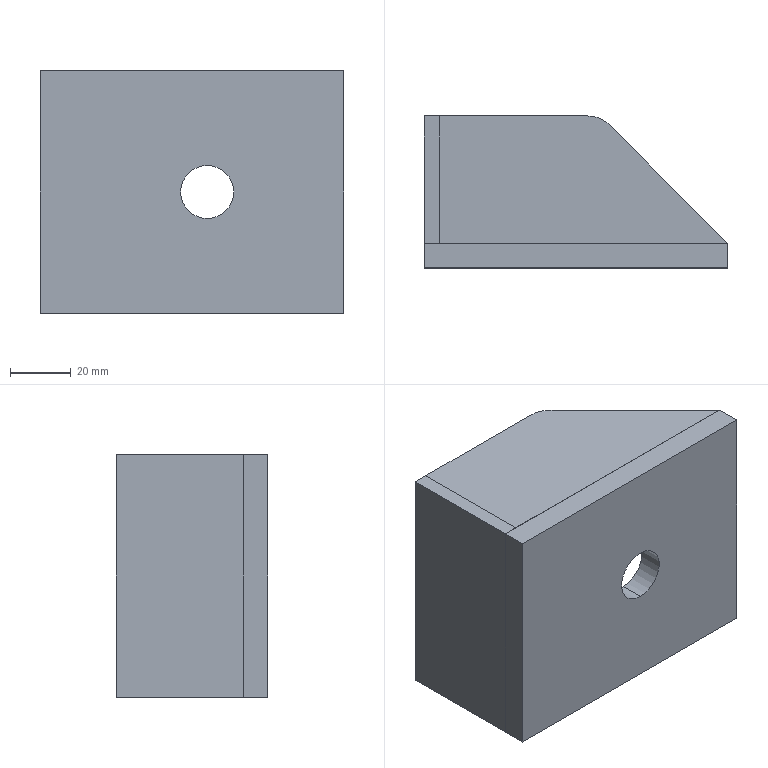Part | STEP file | 2-Foot seat_default<welded> | 4 solids | 28 faces | box 100 x 50 x 80 mm | volume 109934 mm3 | plane 24 | cylinder 4 | commonest cylinder face diameters 17.5 x2 20 x2